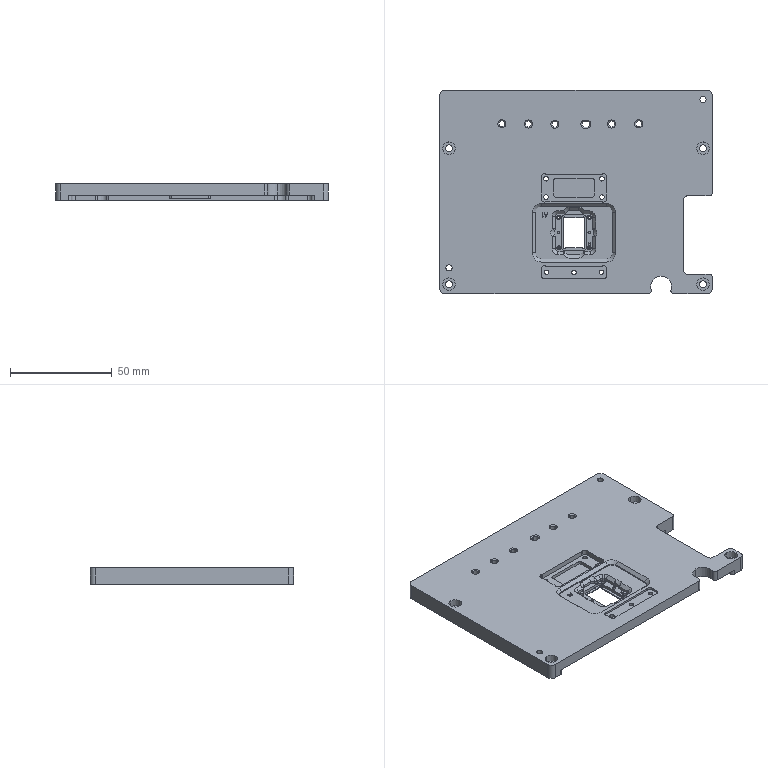NC program | NX | posted with a generic post | part box 134 x 100 x 8 mm
Lines 1 to 1536 of 3418:
N10 G17 G21 G94 G90
(FLOOR_WALL_COPY_COPY , TOOL : D63)
N12 T03 M6
N14 G54
N16 G17 G0 G90 X-101.5 Y49.999 S6500 M3
N18 G43 Z30. H3
N20 Z6.025
N22 G94 G1 Z3.025 F1250.
N24 X-98.5
N26 X98.5
N28 Y12.6
N30 X-98.5
N32 Y-24.8
N34 X98.5
N36 X101.5
N38 Z6.025
N40 G0 Z30.
N42 X-101.5 Y49.999
N44 Z5.05
N46 G1 Z2.05
N48 X-98.5
N50 X98.5
N52 Y12.6
N54 X-98.5
N56 Y-24.8
N58 X98.5
N60 X101.5
N62 Z5.05
N64 G0 Z30.
N66 X-101.5 Y49.999
N68 Z4.075
N70 G1 Z1.075
N72 X-98.5
N74 X98.5
N76 Y12.6
N78 X-98.5
N80 Y-24.8
N82 X98.5
N84 X101.5
N86 Z4.075
N88 G0 Z30.
N90 X-101.5 Y49.999
N92 Z3.1
N94 G1 Z0.1
N96 X-98.5
N98 X98.5
N100 Y12.6
N102 X-98.5
N104 Y-24.8
N106 X98.5
N108 X101.5
N110 Z3.1
N112 G0 Z30.
(FLOOR_WALL_COPY_COPY_1 , TOOL : D63)
N114 X-101.5 Y49.999
N116 Z3.
N118 G1 Z0.
N120 X-98.5
N122 X98.5
N124 Y12.6
N126 X-98.5
N128 Y-24.8
N130 X98.5
N132 X101.5
N134 Z3.
N136 G0 Z30.
N138 M5
(CAVITY_MILL_1 , TOOL : D10)
N140 T04 M6
N142 G54
N144 G17 G0 G90 X4.209 Y-56.998 S9500 M3
N146 G43 Z30. H4
N148 Z0.7
N150 G94 G1 Z-0.8 F1000.
N152 X0.745 Y-50.998
N154 G3 X-0.121 Y-50.498 R1.
N156 G1 Y-8.498
N158 X12.051 F3000.
N160 Y-2.752
N162 X-11.674
N164 G2 X-12.293 Y-8.498 R48.6
N166 G1 X-0.121
N168 Y-15.498
N170 X19.051
N172 Y4.248
N174 X-18.619
N176 Y-0.431
N178 G2 X-21.443 Y-15.498 R41.6
N180 G1 X-0.121
N182 Y-22.498
N184 X26.051
N186 Y11.248
N188 X-25.619
N190 Y-0.431
N192 G2 X-30.082 Y-17.43 R34.6
N194 G1 Y-22.498
N196 X-0.121
N198 Y-29.498
N200 X33.051
N202 Y18.248
N204 X-32.619
N206 Y-0.431
N208 G2 X-37.082 Y-15.48 R27.6
N210 G1 Y-26.915
N212 G2 X-35.594 Y-29.498 R27.6
N214 G1 X-0.121
N216 Y-36.498
N218 X40.051
N220 Y25.248
N222 X-39.619
N224 Y-0.431
N226 G2 X-44.082 Y-13.237 R20.6
N228 G1 Y-29.159
N230 G2 X-40.473 Y-36.091 R20.6
N232 X-38.251 Y-36.498 R14.
N234 G1 X-0.121
N236 Y-43.498
N238 X47.051
N240 Y25.935
N242 G2 X47.492 Y29.404 R13.85
N244 X47.064 Y32.261 R13.85
N246 X44.253 Y32.672 R13.85
N248 X40.855 Y32.248 R13.85
N250 G1 X-40.679
N252 G2 X-44. Y32.652 R13.85
N254 X-46.619 Y32.266 R13.85
N256 G1 Y31.496
N258 G2 X-46.778 Y29.404 R13.85
N260 X-46.619 Y27.311 R13.85
N262 G1 Y-0.431
N264 G2 X-51.082 Y-10.505 R13.6
N266 G1 Y-31.89
N268 G2 X-46.619 Y-41.964 R13.6
N270 G1 Y-43.498
N272 X-44.414
N274 G2 X-39.334 Y-43.498 R7.
N276 G1 X-0.121
N278 Y-50.498
N280 X52.904
N282 G3 X55.984 Y-54.998 R8.
N284 G1 X59.494
N286 G2 X54.051 Y-48.5 R6.6
N288 G1 Y25.935
N290 G2 X54.994 Y29.404 R6.85
N292 X54.051 Y32.873 R6.85
N294 G1 Y39.248
N296 X47.651
N298 G2 X44.253 Y40.15 R6.85
N300 X40.855 Y39.248 R6.85
N302 G1 X-40.679
N304 G2 X-44. Y40.107 R6.85
N306 X-47.322 Y39.248 R6.85
N308 G1 X-53.619
N310 Y31.496
N312 G2 X-53.946 Y29.404 R6.85
N314 X-53.619 Y27.311 R6.85
N316 G1 Y-0.431
N318 G2 X-59.071 Y-6.931 R6.601
N320 G1 X-58.082
N322 Y-35.464
N324 X-58.576
N326 X-59.074
N328 G2 X-53.619 Y-41.964 R6.6
N330 G1 Y-48.5
N332 G2 X-59.062 Y-54.998 R6.6
N334 G1 X-55.552
N336 G3 X-52.472 Y-50.498 R8.
N338 G1 X-42.008
N340 G3 X-41.874 Y-50.021 R6.5
N342 X-41.74 Y-50.498 R6.5
N344 G1 X-0.121
N346 G2 X0.745 Y-50.998 R1.
N348 G1 X4.209 Y-56.998
N350 Z0.7
N352 G0 Z30.
N354 X-22.189 Y8.133
N356 Z0.7
N358 G1 X-20.954 Y9.197 Z0.615 F1000.
N360 X-18.596 Y10.742 Z0.467
N362 X-17.579 Y11.248 Z0.407
N364 X-25.619 Z-0.014
N366 Y4.322 Z-0.377
N368 X-24.967 Y5.253 Z-0.437
N370 X-23.09 Y7.357 Z-0.584
N372 X-20.954 Y9.197 Z-0.732
N374 X-18.596 Y10.742 Z-0.88
N376 X-17.579 Y11.248 Z-0.939
N378 X-21.599 Z-1.15
N380 X-25.619 F3000.
N382 Y4.322
N384 G2 X-17.579 Y11.248 R21.5
N386 G1 X-12.996 Y13.248
N388 X14.996
N390 G3 X14.588 Y10.953 R5.
N392 X10. Y11.5 R19.5
N394 G1 X-8.
N396 G3 X-12.588 Y10.953 R19.5
N398 X-12.996 Y13.248 R5.
N400 G1 X-17.579 Y11.248
N402 X-21.599
N404 Y18.248
N406 X-32.619
N408 Y-0.435
N410 G2 X-35.715 Y-13.133 R27.6
N412 G1 X-29.5 Y-16.354
N414 G2 X-30.082 Y-17.43 R34.6
N416 G1 Y-22.498
N418 X-29.5
N420 Y-16.354
N422 X-29.503 Y-11.354
N424 G3 X-27.619 Y-0.436 R32.6
N426 G1 Y-0.26
N428 G3 X-26.065 Y-0.658 R5.
N430 X-27.5 Y-8. R19.5
N432 G1 Y-11.771
N434 G3 X-29.503 Y-11.354 R5.
N436 G1 X-29.5 Y-16.354
N438 X-35.715 Y-13.133
N440 G2 X-37.082 Y-15.48 R27.6
N442 G1 Y-26.915
N444 G2 X-35.594 Y-29.498 R27.6
N446 G1 X-22.5
N448 Y-8.
N450 G2 X-8. Y6.5 R14.5
N452 G1 X10.
N454 G2 X16.46 Y4.981 R14.5
N456 G1 X19.579 Y11.248
N458 G2 X26.051 Y6.305 R21.5
N460 G1 X27.736 Y0.845
N462 X26.051 Y6.305
N464 Y11.248
N466 X19.579
N468 X16.46 Y4.981
N470 G2 X24.5 Y-8. R14.5
N472 G1 Y-29.498
N474 X33.051
N476 Y18.248
N478 X-21.599
N480 Y25.248
N482 X-39.619
N484 Y-0.434
N486 G2 X-44.082 Y-13.237 R20.6
N488 G1 Y-29.159
N490 G2 X-40.473 Y-36.091 R20.6
N492 X-38.25 Y-36.498 R14.
N494 G1 X-14.002
N496 G2 X-15.5 Y-32. R7.5
N498 G1 Y-8.
N500 G2 X-8. Y-0.5 R7.5
N502 G1 X10.
N504 G2 X17.5 Y-8. R7.5
N506 G1 Y-32.
N508 G2 X16.002 Y-36.498 R7.5
N510 G1 X14.881 Y-35.658
N512 G2 X10. Y-38.1 R6.1
N514 G1 X-8.
N516 G2 X-14.1 Y-32. R6.1
N518 G1 Y-8.
N520 G2 X-8. Y-1.9 R6.1
N522 G1 X10.
N524 G2 X16.1 Y-8. R6.1
N526 G1 Y-32.
N528 G2 X14.881 Y-35.658 R6.1
N530 G1 X16.002 Y-36.498
N532 X40.051
N534 Y25.248
N536 X-21.599
N538 Y32.248
N540 X-40.679
N542 G2 X-44. Y32.652 R13.85
N544 X-46.619 Y32.266 R13.85
N546 G1 Y31.496
N548 G2 X-46.778 Y29.404 R13.85
N550 X-46.619 Y27.311 R13.85
N552 G1 Y-0.433
N554 G2 X-51.082 Y-10.505 R13.6
N556 G1 Y-31.89
N558 G2 X-46.619 Y-41.964 R13.6
N560 G1 Y-43.498
N562 X-44.414
N564 G2 X-39.334 Y-43.498 R7.
N566 G1 X47.051
N568 Y25.934
N570 G2 X47.492 Y29.404 R13.85
N572 X47.064 Y32.261 R13.85
N574 X44.253 Y32.672 R13.85
N576 X40.855 Y32.248 R13.85
N578 G1 X-21.599
N580 Y39.248
N582 X-40.679
N584 G2 X-44. Y40.107 R6.85
N586 X-47.322 Y39.248 R6.85
N588 G1 X-53.619
N590 Y31.496
N592 G2 X-53.946 Y29.404 R6.85
N594 X-53.619 Y27.311 R6.85
N596 G1 Y-0.432
N598 G2 X-59.071 Y-6.931 R6.601
N600 G1 X-58.082
N602 Y-35.464
N604 X-59.074
N606 G2 X-53.619 Y-41.964 R6.6
N608 G1 Y-48.5
N610 G2 X-59.063 Y-54.998 R6.6
N612 G1 X-55.552
N614 G3 X-52.472 Y-50.498 R8.
N616 G1 X-42.008
N618 G3 X-41.874 Y-50.021 R6.5
N620 X-41.74 Y-50.498 R6.5
N622 G1 X52.904
N624 G3 X55.984 Y-54.998 R8.
N626 G1 X59.495
N628 G2 X54.051 Y-48.5 R6.6
N630 G1 Y25.934
N632 G2 X54.994 Y29.404 R6.85
N634 X54.051 Y32.873 R6.85
N636 G1 Y39.248
N638 X47.651
N640 G2 X44.253 Y40.15 R6.85
N642 X40.855 Y39.248 R6.85
N644 G1 X-21.599
N646 G3 X-22.465 Y38.748 R1.
N648 G1 Z0.35
N650 G0 Z30.
N652 X-18.308 Y10.885
N654 Z0.35
N656 G1 X-17.579 Y11.248 Z0.307 F1000.
N658 X-25.619 Z-0.114
N660 Y4.322 Z-0.477
N662 X-24.967 Y5.253 Z-0.537
N664 X-23.09 Y7.357 Z-0.684
N666 X-20.954 Y9.197 Z-0.832
N668 X-18.596 Y10.742 Z-0.98
N670 X-17.579 Y11.248 Z-1.039
N672 X-21.599 Z-1.25
N674 X-25.619 F3000.
N676 Y4.322
N678 G2 X-17.579 Y11.248 R21.5
N680 G1 X-12.996 Y13.248
N682 X14.996
N684 G3 X14.588 Y10.953 R5.
N686 X10. Y11.5 R19.5
N688 G1 X-8.
N690 G3 X-12.588 Y10.953 R19.5
N692 X-12.996 Y13.248 R5.
N694 G1 X-17.579 Y11.248
N696 X-21.599
N698 Y18.248
N700 X-32.619
N702 Y-0.431
N704 G2 X-35.715 Y-13.133 R27.6
N706 G1 X-29.5 Y-16.354
N708 G2 X-30.082 Y-17.43 R34.6
N710 G1 Y-22.498
N712 X-29.5
N714 Y-16.354
N716 X-29.503 Y-11.354
N718 G3 X-27.619 Y-0.431 R32.6
N720 G1 Y-0.26
N722 G3 X-26.065 Y-0.658 R5.
N724 X-27.5 Y-8. R19.5
N726 G1 Y-11.771
N728 G3 X-29.503 Y-11.354 R5.
N730 G1 X-29.5 Y-16.354
N732 X-35.715 Y-13.133
N734 G2 X-37.082 Y-15.48 R27.6
N736 G1 Y-26.915
N738 G2 X-35.594 Y-29.498 R27.6
N740 G1 X-22.5
N742 Y-8.
N744 G2 X-8. Y6.5 R14.5
N746 G1 X10.
N748 G2 X16.46 Y4.981 R14.5
N750 G1 X19.579 Y11.248
N752 G2 X26.051 Y6.305 R21.5
N754 G1 X27.736 Y0.845
N756 X26.051 Y6.305
N758 Y11.248
N760 X19.579
N762 X16.46 Y4.981
N764 G2 X24.5 Y-8. R14.5
N766 G1 Y-29.498
N768 X33.051
N770 Y18.248
N772 X-21.599
N774 Y25.248
N776 X-39.619
N778 Y-0.431
N780 G2 X-44.082 Y-13.237 R20.6
N782 G1 Y-29.159
N784 G2 X-40.473 Y-36.091 R20.6
N786 X-38.25 Y-36.498 R14.
N788 G1 X-14.001
N790 G2 X-15.5 Y-32. R7.5
N792 G1 Y-8.
N794 G2 X-8. Y-0.5 R7.5
N796 G1 X10.
N798 G2 X17.5 Y-8. R7.5
N800 G1 Y-32.
N802 G2 X16.001 Y-36.498 R7.5
N804 G1 X14.881 Y-35.658
N806 G2 X10. Y-38.1 R6.1
N808 G1 X-8.
N810 G2 X-14.1 Y-32. R6.1
N812 G1 Y-8.
N814 G2 X-8. Y-1.9 R6.1
N816 G1 X10.
N818 G2 X16.1 Y-8. R6.1
N820 G1 Y-32.
N822 G2 X14.881 Y-35.658 R6.1
N824 G1 X16.001 Y-36.498
N826 X40.051
N828 Y25.248
N830 X-21.599
N832 Y32.248
N834 X-40.679
N836 G2 X-44. Y32.652 R13.85
N838 X-46.619 Y32.266 R13.85
N840 G1 Y31.496
N842 G2 X-46.778 Y29.404 R13.85
N844 X-46.619 Y27.311 R13.85
N846 G1 Y-0.431
N848 G2 X-51.082 Y-10.505 R13.6
N850 G1 Y-31.89
N852 G2 X-46.619 Y-41.964 R13.6
N854 G1 Y-43.498
N856 X-44.414
N858 G2 X-39.334 Y-43.498 R7.
N860 G1 X47.051
N862 Y25.934
N864 G2 X47.492 Y29.404 R13.85
N866 X47.064 Y32.261 R13.85
N868 X44.253 Y32.672 R13.85
N870 X40.855 Y32.248 R13.85
N872 G1 X-21.599
N874 Y39.248
N876 X-40.679
N878 G2 X-44. Y40.107 R6.85
N880 X-47.322 Y39.248 R6.85
N882 G1 X-53.619
N884 Y31.496
N886 G2 X-53.946 Y29.404 R6.85
N888 X-53.619 Y27.311 R6.85
N890 G1 Y-0.431
N892 G2 X-59.074 Y-6.931 R6.6
N894 G1 X-58.082
N896 Y-34.255
N898 Y-35.464
N900 X-59.074
N902 G2 X-53.619 Y-41.964 R6.6
N904 G1 Y-48.5
N906 G2 X-59.063 Y-54.998 R6.6
N908 G1 X-55.552
N910 G3 X-52.472 Y-50.498 R8.
N912 G1 X-42.008
N914 G3 X-41.874 Y-50.021 R6.5
N916 X-41.74 Y-50.498 R6.5
N918 G1 X52.904
N920 G3 X55.984 Y-54.998 R8.
N922 G1 X59.495
N924 G2 X54.051 Y-48.5 R6.6
N926 G1 Y25.934
N928 G2 X54.994 Y29.404 R6.85
N930 X54.051 Y32.873 R6.85
N932 G1 Y39.248
N934 X47.651
N936 G2 X44.253 Y40.15 R6.85
N938 X40.855 Y39.248 R6.85
N940 G1 X-21.599
N942 G3 X-22.465 Y38.748 R1.
N944 G1 Z0.25
N946 G0 Z30.
N948 X-25.13 Y5.02
N950 Z0.25
N952 G1 X-24.967 Y5.253 Z0.235 F1000.
N954 X-23.09 Y7.357 Z0.087
N956 X-20.954 Y9.197 Z-0.06
N958 X-18.596 Y10.742 Z-0.208
N960 X-17.579 Y11.248 Z-0.268
N962 X-25.619 Z-0.689
N964 Y4.322 Z-1.052
N966 X-24.967 Y5.253 Z-1.112
N968 X-23.09 Y7.357 Z-1.259
N970 X-20.954 Y9.197 Z-1.407
N972 X-18.596 Y10.742 Z-1.555
N974 X-17.579 Y11.248 Z-1.614
N976 X-21.599 Z-1.825
N978 X-25.619 F3000.
N980 Y4.322
N982 G2 X-17.579 Y11.248 R21.5
N984 G1 X-12.996 Y13.248
N986 X14.996
N988 G3 X14.588 Y10.953 R5.
N990 X10. Y11.5 R19.5
N992 G1 X-8.
N994 G3 X-12.588 Y10.953 R19.5
N996 X-12.996 Y13.248 R5.
N998 G1 X-17.579 Y11.248
N1000 X-21.599
N1002 Y18.248
N1004 X-32.619
N1006 Y-0.431
N1008 G2 X-35.715 Y-13.133 R27.6
N1010 G1 X-29.5 Y-16.354
N1012 G2 X-30.082 Y-17.43 R34.6
N1014 G1 Y-22.498
N1016 X-29.5
N1018 Y-16.354
N1020 X-29.503 Y-11.354
N1022 G3 X-27.619 Y-0.431 R32.6
N1024 G1 Y-0.26
N1026 G3 X-26.065 Y-0.658 R5.
N1028 X-27.5 Y-8. R19.5
N1030 G1 Y-11.771
N1032 G3 X-29.503 Y-11.354 R5.
N1034 G1 X-29.5 Y-16.354
N1036 X-35.715 Y-13.133
N1038 G2 X-37.082 Y-15.48 R27.6
N1040 G1 Y-26.915
N1042 G2 X-35.594 Y-29.498 R27.6
N1044 G1 X-22.5
N1046 Y-8.
N1048 G2 X-8. Y6.5 R14.5
N1050 G1 X10.
N1052 G2 X16.46 Y4.981 R14.5
N1054 G1 X19.579 Y11.248
N1056 G2 X26.051 Y6.305 R21.5
N1058 G1 X27.736 Y0.845
N1060 X26.051 Y6.305
N1062 Y11.248
N1064 X19.579
N1066 X16.46 Y4.981
N1068 G2 X24.5 Y-8. R14.5
N1070 G1 Y-29.498
N1072 X33.051
N1074 Y18.248
N1076 X-21.599
N1078 Y25.248
N1080 X-39.619
N1082 Y-0.431
N1084 G2 X-44.082 Y-13.237 R20.6
N1086 G1 Y-29.159
N1088 G2 X-40.473 Y-36.091 R20.6
N1090 X-38.25 Y-36.498 R14.
N1092 G1 X-14.001
N1094 G2 X-15.5 Y-32. R7.5
N1096 G1 Y-8.
N1098 G2 X-8. Y-0.5 R7.5
N1100 G1 X10.
N1102 G2 X17.5 Y-8. R7.5
N1104 G1 Y-32.
N1106 G2 X16.001 Y-36.498 R7.5
N1108 G1 X14.881 Y-35.659
N1110 G2 X10. Y-38.1 R6.1
N1112 G1 X-8.
N1114 G2 X-14.1 Y-32. R6.1
N1116 G1 Y-8.
N1118 G2 X-8. Y-1.9 R6.1
N1120 G1 X10.
N1122 G2 X16.1 Y-8. R6.1
N1124 G1 Y-32.
N1126 G2 X14.881 Y-35.659 R6.1
N1128 G1 X16.001 Y-36.498
N1130 X40.051
N1132 Y25.248
N1134 X-21.599
N1136 Y32.248
N1138 X-40.679
N1140 G2 X-44. Y32.652 R13.85
N1142 X-46.619 Y32.266 R13.85
N1144 G1 Y31.496
N1146 G2 X-46.778 Y29.404 R13.85
N1148 X-46.619 Y27.311 R13.85
N1150 G1 Y-0.431
N1152 G2 X-51.082 Y-10.505 R13.6
N1154 G1 Y-31.89
N1156 G2 X-46.619 Y-41.964 R13.6
N1158 G1 Y-43.498
N1160 X-44.415
N1162 G2 X-39.334 Y-43.498 R7.
N1164 G1 X47.051
N1166 Y25.934
N1168 G2 X47.492 Y29.404 R13.85
N1170 X47.064 Y32.261 R13.85
N1172 X44.253 Y32.672 R13.85
N1174 X40.855 Y32.248 R13.85
N1176 G1 X-21.599
N1178 Y39.248
N1180 X-40.679
N1182 G2 X-44. Y40.107 R6.85
N1184 X-47.322 Y39.248 R6.85
N1186 G1 X-53.619
N1188 Y31.496
N1190 G2 X-53.946 Y29.404 R6.85
N1192 X-53.619 Y27.311 R6.85
N1194 G1 Y-0.431
N1196 G2 X-59.074 Y-6.931 R6.6
N1198 G1 X-58.082
N1200 Y-35.464
N1202 X-59.074
N1204 G2 X-53.619 Y-41.964 R6.6
N1206 G1 Y-48.5
N1208 G2 X-59.064 Y-54.998 R6.6
N1210 G1 X-55.552
N1212 G3 X-52.472 Y-50.498 R8.
N1214 G1 X-42.008
N1216 G3 X-41.874 Y-50.021 R6.5
N1218 X-41.74 Y-50.498 R6.5
N1220 G1 X52.904
N1222 G3 X55.984 Y-54.998 R8.
N1224 G1 X59.496
N1226 G2 X54.051 Y-48.5 R6.6
N1228 G1 Y25.934
N1230 G2 X54.994 Y29.404 R6.85
N1232 X54.051 Y32.873 R6.85
N1234 G1 Y39.248
N1236 X47.651
N1238 G2 X44.253 Y40.15 R6.85
N1240 X40.855 Y39.248 R6.85
N1242 G1 X-21.599
N1244 G3 X-22.465 Y38.748 R1.
N1246 G1 Z-0.325
N1248 G0 X-25.13 Y5.02
N1250 G1 X-24.967 Y5.253 Z-0.34 F1000.
N1252 X-23.09 Y7.357 Z-0.488
N1254 X-20.954 Y9.197 Z-0.635
N1256 X-18.596 Y10.742 Z-0.783
N1258 X-17.579 Y11.248 Z-0.843
N1260 X-25.619 Z-1.264
N1262 Y4.322 Z-1.627
N1264 X-24.967 Y5.253 Z-1.687
N1266 X-23.09 Y7.357 Z-1.834
N1268 X-20.954 Y9.197 Z-1.982
N1270 X-18.596 Y10.742 Z-2.13
N1272 X-17.579 Y11.248 Z-2.189
N1274 X-21.599 Z-2.4
N1276 X-25.619 F3000.
N1278 Y4.322
N1280 G2 X-17.579 Y11.248 R21.5
N1282 G1 X-12.996 Y13.248
N1284 X14.996
N1286 G3 X14.588 Y10.953 R5.
N1288 X10. Y11.5 R19.5
N1290 G1 X-8.
N1292 G3 X-12.588 Y10.953 R19.5
N1294 X-12.996 Y13.248 R5.
N1296 G1 X-17.579 Y11.248
N1298 X-21.599
N1300 Y18.248
N1302 X-32.619
N1304 Y-0.431
N1306 G2 X-35.715 Y-13.133 R27.6
N1308 G1 X-29.5 Y-16.354
N1310 G2 X-30.082 Y-17.43 R34.6
N1312 G1 Y-22.498
N1314 X-29.5
N1316 Y-16.354
N1318 X-29.503 Y-11.354
N1320 G3 X-27.619 Y-0.431 R32.6
N1322 G1 Y-0.26
N1324 G3 X-26.065 Y-0.658 R5.
N1326 X-27.5 Y-8. R19.5
N1328 G1 Y-11.771
N1330 G3 X-29.503 Y-11.354 R5.
N1332 G1 X-29.5 Y-16.354
N1334 X-35.715 Y-13.133
N1336 G2 X-37.082 Y-15.48 R27.6
N1338 G1 Y-26.915
N1340 G2 X-35.594 Y-29.498 R27.6
N1342 G1 X-22.5
N1344 Y-8.
N1346 G2 X-8. Y6.5 R14.5
N1348 G1 X10.
N1350 G2 X16.46 Y4.981 R14.5
N1352 G1 X19.579 Y11.248
N1354 G2 X26.051 Y6.305 R21.5
N1356 G1 X27.736 Y0.845
N1358 X26.051 Y6.305
N1360 Y11.248
N1362 X19.579
N1364 X16.46 Y4.981
N1366 G2 X24.5 Y-8. R14.5
N1368 G1 Y-29.498
N1370 X33.051
N1372 Y18.248
N1374 X-21.599
N1376 Y25.248
N1378 X-39.619
N1380 Y-0.431
N1382 G2 X-44.082 Y-13.237 R20.6
N1384 G1 Y-29.159
N1386 G2 X-40.473 Y-36.091 R20.6
N1388 X-38.249 Y-36.498 R14.
N1390 G1 X-14.001
N1392 G2 X-15.5 Y-32. R7.5
N1394 G1 Y-8.
N1396 G2 X-8. Y-0.5 R7.5
N1398 G1 X10.
N1400 G2 X17.5 Y-8. R7.5
N1402 G1 Y-32.
N1404 G2 X16.001 Y-36.498 R7.5
N1406 G1 X14.881 Y-35.659
N1408 G2 X10. Y-38.1 R6.1
N1410 G1 X-8.
N1412 G2 X-14.1 Y-32. R6.1
N1414 G1 Y-8.
N1416 G2 X-8. Y-1.9 R6.1
N1418 G1 X10.
N1420 G2 X16.1 Y-8. R6.1
N1422 G1 Y-32.
N1424 G2 X14.881 Y-35.659 R6.1
N1426 G1 X16.001 Y-36.498
N1428 X40.051
N1430 Y25.248
N1432 X-21.599
N1434 Y32.248
N1436 X-40.679
N1438 G2 X-44. Y32.652 R13.85
N1440 X-46.619 Y32.266 R13.85
N1442 G1 Y31.496
N1444 G2 X-46.778 Y29.404 R13.85
N1446 X-46.619 Y27.311 R13.85
N1448 G1 Y-0.431
N1450 G2 X-51.082 Y-10.505 R13.6
N1452 G1 Y-31.89
N1454 G2 X-46.619 Y-41.964 R13.6
N1456 G1 Y-43.498
N1458 X-44.415
N1460 G2 X-39.333 Y-43.498 R7.
N1462 G1 X47.051
N1464 Y25.934
N1466 G2 X47.492 Y29.404 R13.85
N1468 X47.064 Y32.261 R13.85
N1470 X44.253 Y32.672 R13.85
N1472 X40.855 Y32.248 R13.85
N1474 G1 X-21.599
N1476 Y39.248
N1478 X-40.679
N1480 G2 X-44. Y40.107 R6.85
N1482 X-47.322 Y39.248 R6.85
N1484 G1 X-53.619
N1486 Y31.496
N1488 G2 X-53.946 Y29.404 R6.85
N1490 X-53.619 Y27.311 R6.85
N1492 G1 Y-0.431
N1494 G2 X-59.071 Y-6.931 R6.601
N1496 G1 X-58.082
N1498 Y-35.464
N1500 X-59.074
N1502 G2 X-53.619 Y-41.964 R6.6
N1504 G1 Y-48.5
N1506 G2 X-59.065 Y-54.998 R6.6
N1508 G1 X-55.553
N1510 G3 X-52.472 Y-50.498 R8.
N1512 G1 X-42.009
N1514 G3 X-41.874 Y-50.021 R6.5
N1516 X-41.74 Y-50.498 R6.5
N1518 G1 X52.904
N1520 G3 X55.985 Y-54.998 R8.
N1522 G1 X59.497
N1524 G2 X54.051 Y-48.5 R6.6
N1526 G1 Y25.934
N1528 G2 X54.994 Y29.404 R6.85
N1530 X54.051 Y32.873 R6.85
N1532 G1 Y39.248
N1534 X47.651
N1536 G2 X44.253 Y40.15 R6.85
N1538 X40.855 Y39.248 R6.85
N1540 G1 X-21.599
N1542 G3 X-22.465 Y38.748 R1.
N1544 G1 Z-0.9
N1546 G0 Z30.
N1548 X0.85 Y-17.401
N1550 Z0.7
N1552 G1 Y-23.913 Z0.359 F1000.
N1554 X0.999 Y-24.004 Z0.35
N1556 X1.15 Y-23.91 Z0.34
N1558 Y-16.092 Z-0.069
N1560 X1. Y-15.995 Z-0.079
N1562 X0.85 Y-16.087 Z-0.088
N1564 Y-23.913 Z-0.498
N1566 X0.999 Y-24.004 Z-0.507
N1568 X1.15 Y-23.91 Z-0.517
N1570 Y-16.092 Z-0.926
N1572 X1. Y-15.995 Z-0.936
N1574 X0.85 Y-16.087 Z-0.945
N1576 Y-20. Z-1.15
N1578 Y-23.913 F3000.
N1580 X0.999 Y-24.004
N1582 X1.15 Y-23.91
N1584 Y-16.092
N1586 X1. Y-15.995
N1588 X0.85 Y-16.087
N1590 Y-20.
N1592 G3 X1.1 Y-20.433 R0.5
N1594 G1 Z0.35
N1596 G0 Z30.
N1598 M5
(CAVITY_MILL_COPY_1 , TOOL : D6JING)
N1600 T16 M6
N1602 G54
N1604 G17 G0 G90 X55.185 Y27.588 S9500 M3
N1606 G43 Z30. H16
N1608 Z-0.45
N1610 G94 G1 X55.852 Y27.614 F1000.
N1612 G3 X56.697 Y28.147 R1.
N1614 G2 X57.656 Y29.404 R4.75 F1800.
N1616 X56.697 Y30.66 R4.75
N1618 G3 X55.852 Y31.194 R1.
N1620 G1 X55.185 Y31.22
N1622 G0 Y27.588 Z-0.9
N1624 G1 X55.852 Y27.614 F1000.
N1626 G3 X56.697 Y28.147 R1.
N1628 G2 X57.656 Y29.404 R4.75 F1800.
N1630 X56.697 Y30.66 R4.75
N1632 G3 X55.852 Y31.194 R1.
N1634 G1 X55.185 Y31.22
N1636 G0 Z30.
N1638 Y27.588
N1640 Z-1.35
N1642 G1 X55.852 Y27.614 F1000.
N1644 G3 X56.697 Y28.147 R1.
N1646 G2 X57.656 Y29.404 R4.75 F1800.
N1648 X56.697 Y30.66 R4.75
N1650 G3 X55.852 Y31.194 R1.
N1652 G1 X55.185 Y31.22
N1654 G0 Y27.588 Z-1.733
N1656 G1 X55.852 Y27.614 F1000.
N1658 G3 X56.697 Y28.147 R1.
N1660 G2 X57.656 Y29.404 R4.75 F1800.
N1662 X56.697 Y30.66 R4.75
N1664 G3 X55.852 Y31.194 R1.
N1666 G1 X55.185 Y31.22
N1668 G0 Y27.588 Z-2.117
N1670 G1 X55.852 Y27.614 F1000.
N1672 G3 X56.697 Y28.147 R1.
N1674 G2 X57.656 Y29.404 R4.75 F1800.
N1676 X56.697 Y30.66 R4.75
N1678 G3 X55.852 Y31.194 R1.
N1680 G1 X55.185 Y31.22
N1682 G0 Y27.588 Z-2.5
N1684 G1 X55.852 Y27.614 F1000.
N1686 G3 X56.697 Y28.147 R1.
N1688 G2 X57.656 Y29.404 R4.75 F1800.
N1690 X56.697 Y30.66 R4.75
N1692 G3 X55.852 Y31.194 R1.
N1694 G1 X55.185 Y31.22
N1696 G0 Z30.
N1698 X54.951 Y37.862
N1700 Z-0.45
N1702 G1 X55.651 Y38.266 F1000.
N1704 G3 X56.151 Y39.132 R1.
N1706 G1 Y41.348 F1800.
N1708 X53.934
N1710 G3 X53.068 Y40.848 R1.
N1712 G1 X52.664 Y40.148
N1714 G0 X54.951 Y37.862 Z-0.9
N1716 G1 X55.651 Y38.266 F1000.
N1718 G3 X56.151 Y39.132 R1.
N1720 G1 Y41.348 F1800.
N1722 X53.934
N1724 G3 X53.068 Y40.848 R1.
N1726 G1 X52.664 Y40.148
N1728 G0 Z30.
N1730 X54.951 Y37.862
N1732 Z-1.35
N1734 G1 X55.651 Y38.266 F1000.
N1736 G3 X56.151 Y39.132 R1.
N1738 G1 Y41.348 F1800.
N1740 X53.934
N1742 G3 X53.068 Y40.848 R1.
N1744 G1 X52.664 Y40.148
N1746 G0 X54.951 Y37.862 Z-1.733
N1748 G1 X55.651 Y38.266 F1000.
N1750 G3 X56.151 Y39.132 R1.
N1752 G1 Y41.348 F1800.
N1754 X53.934
N1756 G3 X53.068 Y40.848 R1.
N1758 G1 X52.664 Y40.148
N1760 G0 X54.951 Y37.862 Z-2.117
N1762 G1 X55.651 Y38.266 F1000.
N1764 G3 X56.151 Y39.132 R1.
N1766 G1 Y41.348 F1800.
N1768 X53.934
N1770 G3 X53.068 Y40.848 R1.
N1772 G1 X52.664 Y40.148
N1774 G0 X54.951 Y37.862 Z-2.5
N1776 G1 X55.651 Y38.266 F1000.
N1778 G3 X56.151 Y39.132 R1.
N1780 G1 Y41.348 F1800.
N1782 X53.934
N1784 G3 X53.068 Y40.848 R1.
N1786 G1 X52.664 Y40.148
N1788 G0 Z30.
N1790 X46.068 Y40.363
N1792 Z-0.45
N1794 G1 X46.034 Y41.029 F1000.
N1796 G3 X45.49 Y41.868 R1.
N1798 G2 X44.29 Y42.742 R4.75 F1800.
N1800 G1 X44.253 Y42.779
N1802 G2 X43.016 Y41.868 R4.75
N1804 G3 X42.472 Y41.029 R1.
N1806 G1 X42.438 Y40.363
N1808 G0 X46.068 Z-0.9
N1810 G1 X46.034 Y41.029 F1000.
N1812 G3 X45.49 Y41.868 R1.
N1814 G2 X44.29 Y42.742 R4.75 F1800.
N1816 G1 X44.253 Y42.779
N1818 G2 X43.016 Y41.868 R4.75
N1820 G3 X42.472 Y41.029 R1.
N1822 G1 X42.438 Y40.363
N1824 G0 Z30.
N1826 X46.068
N1828 Z-1.35
N1830 G1 X46.034 Y41.029 F1000.
N1832 G3 X45.49 Y41.868 R1.
N1834 G2 X44.29 Y42.742 R4.75 F1800.
N1836 G1 X44.253 Y42.779
N1838 G2 X43.016 Y41.868 R4.75
N1840 G3 X42.472 Y41.029 R1.
N1842 G1 X42.438 Y40.363
N1844 G0 X46.068 Z-1.733
N1846 G1 X46.034 Y41.029 F1000.
N1848 G3 X45.49 Y41.868 R1.
N1850 G2 X44.29 Y42.742 R4.75 F1800.
N1852 G1 X44.253 Y42.779
N1854 G2 X43.016 Y41.868 R4.75
N1856 G3 X42.472 Y41.029 R1.
N1858 G1 X42.438 Y40.363
N1860 G0 X46.068 Z-2.117
N1862 G1 X46.034 Y41.029 F1000.
N1864 G3 X45.49 Y41.868 R1.
N1866 G2 X44.253 Y42.779 R4.75 F1800.
N1868 X43.016 Y41.868 R4.75
N1870 G3 X42.472 Y41.029 R1.
N1872 G1 X42.438 Y40.363
N1874 G0 X46.068 Z-2.5
N1876 G1 X46.034 Y41.029 F1000.
N1878 G3 X45.49 Y41.868 R1.
N1880 G2 X44.253 Y42.779 R4.75 F1800.
N1882 X43.016 Y41.868 R4.75
N1884 G3 X42.472 Y41.029 R1.
N1886 G1 X42.438 Y40.363
N1888 G0 Z30.
N1890 X2.05 Y-17.517
N1892 Z-1.25
N1894 G1 X2.75 Y-17.113 F1000.
N1896 G3 X3.25 Y-16.247 R1.
N1898 G1 Y-14.723 F1800.
N1900 G2 X1. Y-13.228 R4.5
N1902 X-1.249 Y-14.723 R4.5
N1904 G1 X-1.25 Y-14.724
N1906 Y-16.246
N1908 G3 X-0.75 Y-17.112 R1.
N1910 G1 X-0.05 Y-17.516
N1912 G0 Z30.
N1914 Y-22.484
N1916 Z-1.25
N1918 G1 X-0.75 Y-22.888 F1000.
N1920 G3 X-1.25 Y-23.754 R1.
N1922 G1 Y-25.277 F1800.
N1924 G2 X1. Y-26.772 R4.5
N1926 X3.25 Y-25.277 R4.5
N1928 G1 Y-23.754
N1930 G3 X2.75 Y-22.888 R1.
N1932 G1 X2.05 Y-22.484
N1934 G0 Z30.
N1936 X-42.187 Y40.342
N1938 Z-0.45
N1940 G1 X-42.23 Y41.008 F1000.
N1942 G3 X-42.784 Y41.84 R1.
N1944 G2 X-44. Y42.703 R4.75 F1800.
N1946 X-45.216 Y41.84 R4.75
N1948 G3 X-45.771 Y41.008 R1.
N1950 G1 X-45.814 Y40.342
N1952 G0 X-42.187 Z-0.9
N1954 G1 X-42.23 Y41.008 F1000.
N1956 G3 X-42.784 Y41.84 R1.
N1958 G2 X-44. Y42.703 R4.75 F1800.
N1960 X-45.216 Y41.84 R4.75
N1962 G3 X-45.771 Y41.008 R1.
N1964 G1 X-45.814 Y40.342
N1966 G0 Z30.
N1968 X-42.187
N1970 Z-1.35
N1972 G1 X-42.23 Y41.008 F1000.
N1974 G3 X-42.784 Y41.84 R1.
N1976 G2 X-44. Y42.703 R4.75 F1800.
N1978 X-45.216 Y41.84 R4.75
N1980 G3 X-45.771 Y41.008 R1.
N1982 G1 X-45.814 Y40.342
N1984 G0 X-42.187 Z-1.733
N1986 G1 X-42.23 Y41.008 F1000.
N1988 G3 X-42.784 Y41.84 R1.
N1990 G2 X-44. Y42.703 R4.75 F1800.
N1992 X-45.216 Y41.84 R4.75
N1994 G3 X-45.771 Y41.008 R1.
N1996 G1 X-45.814 Y40.342
N1998 G0 X-42.187 Z-2.117
N2000 G1 X-42.23 Y41.008 F1000.
N2002 G3 X-42.784 Y41.84 R1.
N2004 G2 X-44. Y42.703 R4.75 F1800.
N2006 X-45.216 Y41.84 R4.75
N2008 G3 X-45.771 Y41.008 R1.
N2010 G1 X-45.814 Y40.342
N2012 G0 X-42.187 Z-2.5
N2014 G1 X-42.23 Y41.008 F1000.
N2016 G3 X-42.784 Y41.84 R1.
N2018 G2 X-44. Y42.703 R4.75 F1800.
N2020 X-45.216 Y41.84 R4.75
N2022 G3 X-45.771 Y41.008 R1.
N2024 G1 X-45.814 Y40.342
N2026 G0 Z30.
N2028 X-52.232 Y40.148
N2030 Z-0.45
N2032 G1 X-52.636 Y40.848 F1000.
N2034 G3 X-53.502 Y41.348 R1.
N2036 G1 X-55.719 F1800.
N2038 Y39.132
N2040 G3 X-55.219 Y38.266 R1.
N2042 G1 X-54.519 Y37.862
N2044 G0 X-52.232 Y40.148 Z-0.9
N2046 G1 X-52.636 Y40.848 F1000.
N2048 G3 X-53.502 Y41.348 R1.
N2050 G1 X-55.719 F1800.
N2052 Y39.132
N2054 G3 X-55.219 Y38.266 R1.
N2056 G1 X-54.519 Y37.862
N2058 G0 Z30.
N2060 X-52.232 Y40.148
N2062 Z-1.35
N2064 G1 X-52.636 Y40.848 F1000.
N2066 G3 X-53.502 Y41.348 R1.
N2068 G1 X-55.719 F1800.
N2070 Y39.132
N2072 G3 X-55.219 Y38.266 R1.
N2074 G1 X-54.519 Y37.862
N2076 G0 X-52.232 Y40.148 Z-1.733
N2078 G1 X-52.636 Y40.848 F1000.
N2080 G3 X-53.502 Y41.348 R1.
N2082 G1 X-55.719 F1800.
N2084 Y39.132
N2086 G3 X-55.219 Y38.266 R1.
N2088 G1 X-54.519 Y37.862
N2090 G0 X-52.232 Y40.148 Z-2.117
N2092 G1 X-52.636 Y40.848 F1000.
N2094 G3 X-53.502 Y41.348 R1.
N2096 G1 X-55.719 F1800.
N2098 Y39.132
N2100 G3 X-55.219 Y38.266 R1.
N2102 G1 X-54.519 Y37.862
N2104 G0 X-52.232 Y40.148 Z-2.5
N2106 G1 X-52.636 Y40.848 F1000.
N2108 G3 X-53.502 Y41.348 R1.
N2110 G1 X-55.719 F1800.
N2112 Y39.132
N2114 G3 X-55.219 Y38.266 R1.
N2116 G1 X-54.519 Y37.862
N2118 G0 Z30.
N2120 X-54.528 Y31.158
N2122 Z-0.45
N2124 G1 X-55.172 Y30.984 F1000.
N2126 G3 X-55.878 Y30.275 R1.
N2128 G2 X-56.204 Y29.404 R4.75 F1800.
N2130 X-55.878 Y28.532 R4.75
N2132 G3 X-55.172 Y27.824 R1.
N2134 G1 X-54.528 Y27.65
N2136 G0 Y31.158 Z-0.9
N2138 G1 X-55.172 Y30.984 F1000.
N2140 G3 X-55.878 Y30.275 R1.
N2142 G2 X-56.204 Y29.404 R4.75 F1800.
N2144 X-55.878 Y28.532 R4.75
N2146 G3 X-55.172 Y27.824 R1.
N2148 G1 X-54.528 Y27.65
N2150 G0 Z30.
N2152 Y31.158
N2154 Z-1.35
N2156 G1 X-55.172 Y30.984 F1000.
N2158 G3 X-55.878 Y30.275 R1.
N2160 G2 X-56.204 Y29.404 R4.75 F1800.
N2162 X-55.878 Y28.532 R4.75
N2164 G3 X-55.172 Y27.824 R1.
N2166 G1 X-54.528 Y27.65
N2168 G0 Y31.158 Z-1.733
N2170 G1 X-55.172 Y30.984 F1000.
N2172 G3 X-55.878 Y30.275 R1.
N2174 G2 X-56.204 Y29.404 R4.75 F1800.
N2176 X-55.878 Y28.532 R4.75
N2178 G3 X-55.172 Y27.824 R1.
N2180 G1 X-54.528 Y27.65
N2182 G0 Y31.158 Z-2.117
N2184 G1 X-55.172 Y30.984 F1000.
N2186 G3 X-55.878 Y30.275 R1.
N2188 G2 X-56.204 Y29.404 R4.75 F1800.
N2190 X-55.878 Y28.532 R4.75
N2192 G3 X-55.172 Y27.824 R1.
N2194 G1 X-54.528 Y27.65
N2196 G0 Y31.158 Z-2.5
N2198 G1 X-55.172 Y30.984 F1000.
N2200 G3 X-55.878 Y30.275 R1.
N2202 G2 X-56.204 Y29.404 R4.75 F1800.
N2204 X-55.878 Y28.532 R4.75
N2206 G3 X-55.172 Y27.824 R1.
N2208 G1 X-54.528 Y27.65
N2210 G0 Z30.
(FLOOR_WALL_COPY_1 , TOOL : D6JING)
N2212 X-9.72 Y-36.695
N2214 Z0.1
N2216 G1 Z-0.9 F1250.
N2218 X-9.241 Y-36.41
N2220 G3 X-8.948 Y-35.886 R0.6
N2222 G1 X-9.371 Y-4.242
N2224 G2 X-8. Y-4. R4.
N2226 G1 X-6.388
N2228 X-5.96 Y-36.
N2230 X-2.973
N2232 X-3.401 Y-4.
N2234 X-0.414
N2236 X0.014 Y-36.
N2238 X3.001
N2240 X2.573 Y-4.
N2242 X5.559
N2244 X5.988 Y-36.
N2246 X8.974
N2248 X8.546 Y-4.
N2250 G3 X8.239 Y-3.484 R0.6
N2252 G1 X7.374 Y-3.
N2254 Z0.1
N2256 G0 Z30.
N2258 X-51.313 Y39.364
N2260 Z-1.4
N2262 G1 X-55.419 Z-2.5
N2264 Y41.048
N2266 X-47.322
N2268 G3 X-44. Y42.294 R5.05
N2270 X-40.679 Y41.048 R5.05
N2272 G1 X40.855
N2274 G3 X44.253 Y42.362 R5.05
N2276 X47.651 Y41.048 R5.05
N2278 G1 X55.851
N2280 Y39.364
N2282 X-55.419
N2284 Y36.365
N2286 X55.851
N2288 Y33.366
N2290 X-55.419
N2292 Y31.496
N2294 G2 X-55.546 Y30.367 R5.05
N2296 G1 X56.516
N2298 G3 X57.231 Y29.404 R5.05
N2300 X56.059 Y27.369 R5.05
N2302 G1 X-55.419
N2304 Y27.311
N2306 Y24.37
N2308 X55.851
N2310 Y21.371
N2312 X-55.419
N2314 Y18.372
N2316 X55.851
N2318 Y15.374
N2320 X-55.419
N2322 Y12.375
N2324 X55.851
N2326 Y9.376
N2328 X-55.419
N2330 Y6.377
N2332 X55.851
N2334 Y3.379
N2336 X-55.419
N2338 Y0.38
N2340 X55.851
N2342 Y-2.619
N2344 X-55.946
N2346 G2 X-58.548 Y-4.931 R4.8
N2348 G1 X-56.082
N2350 Y-5.618
N2352 X-11.58
N2354 G3 X-12.3 Y-8. R4.3
N2356 G1 Y-8.616
N2358 X-56.082
N2360 Y-11.615
N2362 X-12.3
N2364 Y-14.614
N2366 X-56.082
N2368 Y-17.613
N2370 X-12.3
N2372 Y-20.611
N2374 X-56.082
N2376 Y-23.61
N2378 X-12.3
N2380 Y-26.609
N2382 X-56.082
N2384 Y-29.608
N2386 X-12.3
N2388 Y-32.
N2390 G3 X-12.257 Y-32.606 R4.3
N2392 G1 X-56.082
N2394 Y-35.605
N2396 X-10.344
N2398 G3 X-10.943 Y-35.573 R0.6
N2400 G1 Z-1.5
N2402 G0 Z30.
N2404 X-11.58 Y-5.618
N2406 Z-1.5
N2408 G1 Z-2.5
N2410 G2 X-8. Y-3.7 R4.3
N2412 G1 X10.
N2414 G2 X13.58 Y-5.618 R4.3
N2416 G1 X55.851
N2418 Y-8.616
N2420 X14.3
N2422 Y-11.615
N2424 X55.851
N2426 Y-14.614
N2428 X14.3
N2430 Y-17.613
N2432 X55.851
N2434 Y-20.611
N2436 X14.3
N2438 Y-23.61
N2440 X55.851
N2442 Y-26.609
N2444 X14.3
N2446 Y-29.608
N2448 X55.851
N2450 Y-32.606
N2452 X14.257
N2454 G2 X12.344 Y-35.605 R4.3
N2456 G1 X55.851
N2458 Y-38.604
N2460 X-56.791
N2462 G2 X-55.432 Y-41.602 R4.8
N2464 G1 X55.851
N2466 Y-44.601
N2468 X-55.419
N2470 Y-47.6
N2472 X55.851
N2474 Y-48.5
N2476 G3 X56.334 Y-50.599 R4.8
N2478 G1 X-55.902
N2480 Z-1.5
N2482 G0 Z30.
N2484 X-60.75 Y-36.464
N2486 Z-1.5
N2488 G1 Z-2.5
N2490 X-60.417 Y-37.14
N2492 G3 X-59.919 Y-37.474 R0.6
N2494 G2 X-55.719 Y-41.964 R4.5
N2496 G1 Y-48.5
N2498 G2 X-59.919 Y-52.99 R4.5
N2500 G3 X-60.417 Y-53.324 R0.6
N2502 G1 X-60.75 Y-54.
N2504 Z-1.5
N2506 G0 Z30.
N2508 X61.182
N2510 Z-1.5
N2512 G1 Z-2.5
N2514 X60.849 Y-53.324
N2516 G3 X60.351 Y-52.99 R0.6
N2518 G2 X56.151 Y-48.5 R4.5
N2520 G1 Y25.934
N2522 G2 X57.656 Y29.404 R4.75
N2524 X56.151 Y32.873 R4.75
N2526 G1 Y41.348
N2528 X47.651
N2530 G2 X44.253 Y42.779 R4.75
N2532 X40.855 Y41.348 R4.75
N2534 G1 X-40.679
N2536 G2 X-44. Y42.703 R4.75
N2538 X-47.322 Y41.348 R4.75
N2540 G1 X-55.719
N2542 Y31.496
N2544 G2 X-56.204 Y29.404 R4.75
N2546 X-55.719 Y27.311 R4.75
N2548 G1 Y-0.431
N2550 G2 X-59.919 Y-4.921 R4.5
N2552 G3 X-60.417 Y-5.255 R0.6
N2554 G1 X-60.75 Y-5.931
N2556 Z-1.5
N2558 G0 Z30.
N2560 X-13.3 Y-21.097
N2562 Z-1.5
N2564 G1 Z-2.5
N2566 X-12.3 Y-20.52
N2568 G3 X-12. Y-20. R0.6
N2570 G1 Y-8.
N2572 G2 X-8. Y-4. R4.
N2574 G1 X10.
N2576 G2 X14. Y-8. R4.
N2578 G1 Y-32.
N2580 G2 X10. Y-36. R4.
N2582 G1 X-8.
N2584 G2 X-12. Y-32. R4.
N2586 G1 Y-20.
N2588 G3 X-12.3 Y-19.48 R0.6
N2590 G1 X-13.3 Y-18.903
N2592 Z-1.5
N2594 G0 Z30.
N2596 M5
(HOLE_MILLING_1_1 , TOOL : D3)
N2598 T18 M6
N2600 G54
N2602 G17 G0 G90 X-12.75 Y6.5 S9500 M3
N2604 G43 Z30. H18
N2606 Z-2.
N2608 G94 G3 X-13. Y6.75 R0.25 F1100.
N2610 X-13.25 Y6.5 R0.25
N2612 X-13.25 Y6.5 Z-2.25 I0.5 J0.
N2614 X-13.25 Y6.5 Z-2.5 I0.5 J0.
N2616 X-13.25 Y6.5 Z-2.75 I0.5 J0.
N2618 X-13.25 Y6.5 Z-3. I0.5 J0.
N2620 X-13.25 Y6.5 Z-3.25 I0.5 J0.
N2622 X-13.25 Y6.5 Z-3.5 I0.5 J0.
N2624 X-13.25 Y6.5 Z-3.75 I0.5 J0.
N2626 X-12.345 Y6.794 Z-3.9 R-0.5
N2628 X-13.044 Y6.905 R0.5
N2630 X-12.345 Y6.794 R-0.5
N2632 X-12.695 Y6.849 R0.25
N2634 X-12.75 Y6.5 R0.25
N2636 G0 Z30.
N2638 Y-2.5
N2640 Z-2.
N2642 G3 X-13. Y-2.25 R0.25
N2644 X-13.25 Y-2.5 R0.25
N2646 X-13.25 Y-2.5 Z-2.25 I0.5 J0.
N2648 X-13.25 Y-2.5 Z-2.5 I0.5 J0.
N2650 X-13.25 Y-2.5 Z-2.75 I0.5 J0.
N2652 X-13.25 Y-2.5 Z-3. I0.5 J0.
N2654 X-13.25 Y-2.5 Z-3.25 I0.5 J0.
N2656 X-13.25 Y-2.5 Z-3.5 I0.5 J0.
N2658 X-13.25 Y-2.5 Z-3.75 I0.5 J0.
N2660 X-12.345 Y-2.206 Z-3.9 R-0.5
N2662 X-13.044 Y-2.095 R0.5
N2664 X-12.345 Y-2.206 R-0.5
N2666 X-12.695 Y-2.151 R0.25
N2668 X-12.75 Y-2.5 R0.25
N2670 G0 Z30.
N2672 X14.75 Y6.5
N2674 Z-2.
N2676 G3 X14.5 Y6.75 R0.25
N2678 X14.25 Y6.5 R0.25
N2680 X14.25 Y6.5 Z-2.25 I0.5 J0.
N2682 X14.25 Y6.5 Z-2.5 I0.5 J0.
N2684 X14.25 Y6.5 Z-2.75 I0.5 J0.
N2686 X14.25 Y6.5 Z-3. I0.5 J0.
N2688 X14.25 Y6.5 Z-3.25 I0.5 J0.
N2690 X14.25 Y6.5 Z-3.5 I0.5 J0.
N2692 X14.25 Y6.5 Z-3.75 I0.5 J0.
N2694 X15.155 Y6.794 Z-3.9 R-0.5
N2696 X14.456 Y6.905 R0.5
N2698 X15.155 Y6.794 R-0.5
N2700 X14.805 Y6.849 R0.25
N2702 X14.75 Y6.5 R0.25
N2704 G0 Z30.
N2706 Y-2.5
N2708 Z-2.
N2710 G3 X14.5 Y-2.25 R0.25
N2712 X14.25 Y-2.5 R0.25
N2714 X14.25 Y-2.5 Z-2.25 I0.5 J0.
N2716 X14.25 Y-2.5 Z-2.5 I0.5 J0.
N2718 X14.25 Y-2.5 Z-2.75 I0.5 J0.
N2720 X14.25 Y-2.5 Z-3. I0.5 J0.
N2722 X14.25 Y-2.5 Z-3.25 I0.5 J0.
N2724 X14.25 Y-2.5 Z-3.5 I0.5 J0.
N2726 X14.25 Y-2.5 Z-3.75 I0.5 J0.
N2728 X15.155 Y-2.206 Z-3.9 R-0.5
N2730 X14.456 Y-2.095 R0.5
N2732 X15.155 Y-2.206 R-0.5
N2734 X14.805 Y-2.151 R0.25
N2736 X14.75 Y-2.5 R0.25
N2738 G0 Z30.
N2740 X14.5 Y-39.5
N2742 Z-2.
N2744 G3 X14.2 Y-39.2 R0.3
N2746 X13.9 Y-39.5 R0.3
N2748 X13.9 Y-39.5 Z-2.25 I0.6 J0.
N2750 X13.9 Y-39.5 Z-2.5 I0.6 J0.
N2752 X13.9 Y-39.5 Z-2.75 I0.6 J0.
N2754 X13.9 Y-39.5 Z-3. I0.6 J0.
N2756 X13.9 Y-39.5 Z-3.25 I0.6 J0.
N2758 X13.9 Y-39.5 Z-3.5 I0.6 J0.
N2760 X13.9 Y-39.5 Z-3.75 I0.6 J0.
N2762 X13.9 Y-39.5 Z-4. I0.6 J0.
N2764 X13.9 Y-39.5 Z-4.25 I0.6 J0.
N2766 X13.9 Y-39.5 Z-4.5 I0.6 J0.
N2768 X13.9 Y-39.5 Z-4.75 I0.6 J0.
N2770 X13.9 Y-39.5 Z-5. I0.6 J0.
N2772 X13.9 Y-39.5 Z-5.25 I0.6 J0.
N2774 X13.9 Y-39.5 Z-5.5 I0.6 J0.
N2776 X14.5 Y-40.1 R0.6
N2778 X13.9 Y-39.5 R-0.6
N2780 X14.2 Y-39.8 R0.3
N2782 X14.5 Y-39.5 R0.3
N2784 G0 Z30.
N2786 X1.
N2788 Z-2.
N2790 G3 X0.7 Y-39.2 R0.3
N2792 X0.4 Y-39.5 R0.3
N2794 X0.4 Y-39.5 Z-2.25 I0.6 J0.
N2796 X0.4 Y-39.5 Z-2.5 I0.6 J0.
N2798 X0.4 Y-39.5 Z-2.75 I0.6 J0.
N2800 X0.4 Y-39.5 Z-3. I0.6 J0.
N2802 X0.4 Y-39.5 Z-3.25 I0.6 J0.
N2804 X0.4 Y-39.5 Z-3.5 I0.6 J0.
N2806 X0.4 Y-39.5 Z-3.75 I0.6 J0.
N2808 X0.4 Y-39.5 Z-4. I0.6 J0.
N2810 X0.4 Y-39.5 Z-4.25 I0.6 J0.
N2812 X0.4 Y-39.5 Z-4.5 I0.6 J0.
N2814 X0.4 Y-39.5 Z-4.75 I0.6 J0.
N2816 X0.4 Y-39.5 Z-5. I0.6 J0.
N2818 X0.4 Y-39.5 Z-5.25 I0.6 J0.
N2820 X0.4 Y-39.5 Z-5.5 I0.6 J0.
N2822 X1. Y-40.1 R0.6
N2824 X0.4 Y-39.5 R-0.6
N2826 X0.7 Y-39.8 R0.3
N2828 X1. Y-39.5 R0.3
N2830 G0 Z30.
N2832 X-12.5
N2834 Z-2.
N2836 G3 X-12.8 Y-39.2 R0.3
N2838 X-13.1 Y-39.5 R0.3
N2840 X-13.1 Y-39.5 Z-2.25 I0.6 J0.
N2842 X-13.1 Y-39.5 Z-2.5 I0.6 J0.
N2844 X-13.1 Y-39.5 Z-2.75 I0.6 J0.
N2846 X-13.1 Y-39.5 Z-3. I0.6 J0.
N2848 X-13.1 Y-39.5 Z-3.25 I0.6 J0.
N2850 X-13.1 Y-39.5 Z-3.5 I0.6 J0.
N2852 X-13.1 Y-39.5 Z-3.75 I0.6 J0.
N2854 X-13.1 Y-39.5 Z-4. I0.6 J0.
N2856 X-13.1 Y-39.5 Z-4.25 I0.6 J0.
N2858 X-13.1 Y-39.5 Z-4.5 I0.6 J0.
N2860 X-13.1 Y-39.5 Z-4.75 I0.6 J0.
N2862 X-13.1 Y-39.5 Z-5. I0.6 J0.
N2864 X-13.1 Y-39.5 Z-5.25 I0.6 J0.
N2866 X-13.1 Y-39.5 Z-5.5 I0.6 J0.
N2868 X-12.5 Y-40.1 R0.6
N2870 X-13.1 Y-39.5 R-0.6
N2872 X-12.8 Y-39.8 R0.3
N2874 X-12.5 Y-39.5 R0.3
N2876 G0 Z30.
(ZLEVEL_PROFILE_COPY_COPY_COPY_1_COPY_COPY_1_COPY_COPY_COPY_1_COPY_COPY_1 , TOO)
N2878 X1.504 Y-28.441
N2880 Z0.6
N2882 G1 X1.511 Y-28.442 F1000.
N2884 X1.705 Y-28.511 Z0.589
N2886 X1.794 Y-28.283 Z0.576
N2888 X2.123 Y-27.754 Z0.543
N2890 X2.553 Y-27.304 Z0.511
N2892 X3.067 Y-26.953 Z0.478
N2894 X3.643 Y-26.715 Z0.445
N2896 X4.255 Y-26.6 Z0.413
N2898 X4.5 Z0.4
N2900 X4.861 Z0.381
N2902 X4.795 Y-26.411 Z0.371
N2904 X4.75 Y-26.144 Z0.356
N2906 Y-13.856 Z-0.288
N2908 X4.795 Y-13.589 Z-0.302
N2910 X4.861 Y-13.4 Z-0.312
N2912 X4.255 Z-0.344
N2914 X3.643 Y-13.285 Z-0.377
N2916 X3.067 Y-13.047 Z-0.409
N2918 X2.553 Y-12.696 Z-0.442
N2920 X2.123 Y-12.246 Z-0.475
N2922 X1.794 Y-11.717 Z-0.507
N2924 X1.705 Y-11.489 Z-0.52
N2926 X1.511 Y-11.558 Z-0.531
N2928 X1.213 Y-11.609 Z-0.547
N2930 X0.802 Y-11.611 Z-0.568
N2932 X0.49 Y-11.558 Z-0.585
N2934 X0.295 Y-11.489 Z-0.596
N2936 X0.206 Y-11.718 Z-0.608
N2938 X-0.123 Y-12.246 Z-0.641
N2940 X-0.553 Y-12.696 Z-0.674
N2942 X-1.067 Y-13.047 Z-0.706
N2944 X-1.643 Y-13.285 Z-0.739
N2946 X-2.255 Y-13.4 Z-0.772
N2948 X-2.861 Z-0.803
N2950 X-2.795 Y-13.589 Z-0.814
N2952 X-2.75 Y-13.856 Z-0.828
N2954 Y-20. Z-1.15
N2956 Y-25.944 F1100.
N2958 G2 X-2.861 Y-26.6 R2.
N2960 G1 X-2.5
N2962 G2 X0.295 Y-28.511 R3.
N2964 X1.705 Y-28.511 R2.11
N2966 X4.5 Y-26.6 R3.
N2968 G1 X4.86
N2970 G2 X4.75 Y-25.944 R2.
N2972 G1 Y-14.056
N2974 G2 X4.861 Y-13.4 R2.
N2976 G1 X4.5
N2978 G2 X1.705 Y-11.489 R3.
N2980 X1.008 Y-11.61 R2.11
N2982 X0.295 Y-11.489 R2.11
N2984 X-2.5 Y-13.4 R3.
N2986 G1 X-2.861
N2988 G2 X-2.75 Y-14.056 R2.
N2990 G1 Y-20.
N2992 Y-25.729 Z-1.25
N2994 Y-25.944
N2996 G2 X-2.861 Y-26.6 R2.
N2998 G1 X-2.5
N3000 G2 X0.295 Y-28.511 R3.
N3002 X1.705 Y-28.511 R2.11
N3004 X4.5 Y-26.6 R3.
N3006 G1 X4.86
N3008 G2 X4.75 Y-25.944 R2.
N3010 G1 Y-14.056
N3012 G2 X4.861 Y-13.4 R2.
N3014 G1 X4.5
N3016 G2 X1.705 Y-11.489 R3.
N3018 X1.008 Y-11.61 R2.11
N3020 X0.295 Y-11.489 R2.11
N3022 X-2.5 Y-13.4 R3.
N3024 G1 X-2.861
N3026 G2 X-2.75 Y-14.056 R2.
N3028 G1 Y-25.729
N3030 Z0.25
N3032 G0 Z30.
N3034 M5